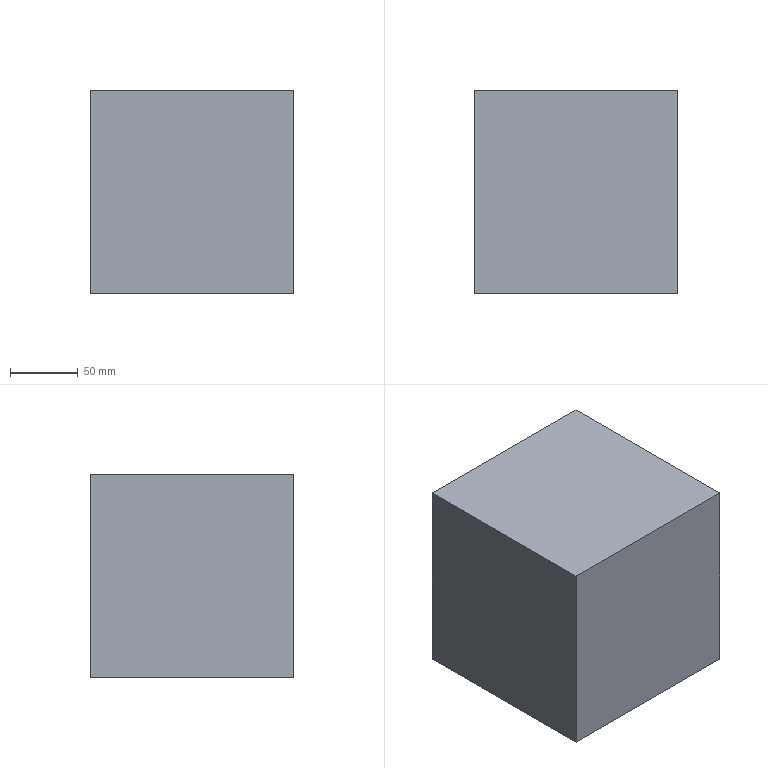Part | STEP file | Collection box | 1 solid | 11 faces | box 150 x 150 x 150 mm | volume 220232 mm3 | plane 11
STEP:
#1=CARTESIAN_POINT('',(75.,75.,-75.));
#2=VERTEX_POINT('',#1);
#3=CARTESIAN_POINT('',(-75.,75.,-75.));
#4=VERTEX_POINT('',#3);
#5=CARTESIAN_POINT('',(-75.,75.,-75.));
#6=DIRECTION('',(-1.,0.,0.));
#7=VECTOR('',#6,1000.);
#8=LINE('',#5,#7);
#9=EDGE_CURVE('',#2,#4,#8,.T.);
#10=ORIENTED_EDGE('',*,*,#9,.T.);
#11=CARTESIAN_POINT('',(-75.,75.,75.));
#12=VERTEX_POINT('',#11);
#13=CARTESIAN_POINT('',(-75.,75.,75.));
#14=DIRECTION('',(0.,0.,-1.));
#15=VECTOR('',#14,1000.);
#16=LINE('',#13,#15);
#17=EDGE_CURVE('',#12,#4,#16,.T.);
#18=ORIENTED_EDGE('',*,*,#17,.F.);
#19=CARTESIAN_POINT('',(75.,75.,75.));
#20=VERTEX_POINT('',#19);
#21=CARTESIAN_POINT('',(-75.,75.,75.));
#22=DIRECTION('',(-1.,0.,0.));
#23=VECTOR('',#22,1000.);
#24=LINE('',#21,#23);
#25=EDGE_CURVE('',#20,#12,#24,.T.);
#26=ORIENTED_EDGE('',*,*,#25,.F.);
#27=CARTESIAN_POINT('',(75.,75.,75.));
#28=DIRECTION('',(0.,0.,-1.));
#29=VECTOR('',#28,1000.);
#30=LINE('',#27,#29);
#31=EDGE_CURVE('',#20,#2,#30,.T.);
#32=ORIENTED_EDGE('',*,*,#31,.T.);
#33=EDGE_LOOP('',(#10,#18,#26,#32));
#34=FACE_OUTER_BOUND('',#33,.T.);
#35=CARTESIAN_POINT('',(73.,75.,-73.));
#36=VERTEX_POINT('',#35);
#37=CARTESIAN_POINT('',(-73.,75.,-73.));
#38=VERTEX_POINT('',#37);
#39=CARTESIAN_POINT('',(0.,75.,-73.));
#40=DIRECTION('',(-1.,0.,0.));
#41=VECTOR('',#40,1000.);
#42=LINE('',#39,#41);
#43=EDGE_CURVE('',#36,#38,#42,.T.);
#44=ORIENTED_EDGE('',*,*,#43,.F.);
#45=CARTESIAN_POINT('',(73.,75.,73.));
#46=VERTEX_POINT('',#45);
#47=CARTESIAN_POINT('',(73.,75.,75.));
#48=DIRECTION('',(0.,0.,-1.));
#49=VECTOR('',#48,1000.);
#50=LINE('',#47,#49);
#51=EDGE_CURVE('',#46,#36,#50,.T.);
#52=ORIENTED_EDGE('',*,*,#51,.F.);
#53=CARTESIAN_POINT('',(-73.,75.,73.));
#54=VERTEX_POINT('',#53);
#55=CARTESIAN_POINT('',(0.,75.,73.));
#56=DIRECTION('',(-1.,0.,0.));
#57=VECTOR('',#56,1000.);
#58=LINE('',#55,#57);
#59=EDGE_CURVE('',#46,#54,#58,.T.);
#60=ORIENTED_EDGE('',*,*,#59,.T.);
#61=CARTESIAN_POINT('',(-73.,75.,75.));
#62=DIRECTION('',(0.,0.,-1.));
#63=VECTOR('',#62,1000.);
#64=LINE('',#61,#63);
#65=EDGE_CURVE('',#54,#38,#64,.T.);
#66=ORIENTED_EDGE('',*,*,#65,.T.);
#67=EDGE_LOOP('',(#44,#52,#60,#66));
#68=FACE_BOUND('',#67,.T.);
#69=CARTESIAN_POINT('',(-75.,75.,75.));
#70=DIRECTION('',(0.,-1.,0.));
#71=DIRECTION('',(0.,0.,-1.));
#72=AXIS2_PLACEMENT_3D('',#69,#70,#71);
#73=PLANE('',#72);
#74=ADVANCED_FACE('',(#34,#68),#73,.F.);
#75=CARTESIAN_POINT('',(75.,-75.,-75.));
#76=VERTEX_POINT('',#75);
#77=CARTESIAN_POINT('',(75.,-75.,-75.));
#78=DIRECTION('',(0.,1.,0.));
#79=VECTOR('',#78,1000.);
#80=LINE('',#77,#79);
#81=EDGE_CURVE('',#76,#2,#80,.T.);
#82=ORIENTED_EDGE('',*,*,#81,.T.);
#83=ORIENTED_EDGE('',*,*,#31,.F.);
#84=CARTESIAN_POINT('',(75.,-75.,75.));
#85=VERTEX_POINT('',#84);
#86=CARTESIAN_POINT('',(75.,-75.,75.));
#87=DIRECTION('',(0.,1.,0.));
#88=VECTOR('',#87,1000.);
#89=LINE('',#86,#88);
#90=EDGE_CURVE('',#85,#20,#89,.T.);
#91=ORIENTED_EDGE('',*,*,#90,.F.);
#92=CARTESIAN_POINT('',(75.,-75.,75.));
#93=DIRECTION('',(0.,0.,-1.));
#94=VECTOR('',#93,1000.);
#95=LINE('',#92,#94);
#96=EDGE_CURVE('',#85,#76,#95,.T.);
#97=ORIENTED_EDGE('',*,*,#96,.T.);
#98=EDGE_LOOP('',(#82,#83,#91,#97));
#99=FACE_OUTER_BOUND('',#98,.T.);
#100=CARTESIAN_POINT('',(75.,-75.,75.));
#101=DIRECTION('',(-1.,0.,0.));
#102=DIRECTION('',(0.,0.,1.));
#103=AXIS2_PLACEMENT_3D('',#100,#101,#102);
#104=PLANE('',#103);
#105=ADVANCED_FACE('',(#99),#104,.F.);
#106=CARTESIAN_POINT('',(-75.,-75.,-75.));
#107=VERTEX_POINT('',#106);
#108=CARTESIAN_POINT('',(-75.,-75.,-75.));
#109=DIRECTION('',(0.,-1.,0.));
#110=VECTOR('',#109,1000.);
#111=LINE('',#108,#110);
#112=EDGE_CURVE('',#4,#107,#111,.T.);
#113=ORIENTED_EDGE('',*,*,#112,.T.);
#114=CARTESIAN_POINT('',(-75.,-75.,75.));
#115=VERTEX_POINT('',#114);
#116=CARTESIAN_POINT('',(-75.,-75.,75.));
#117=DIRECTION('',(0.,0.,-1.));
#118=VECTOR('',#117,1000.);
#119=LINE('',#116,#118);
#120=EDGE_CURVE('',#115,#107,#119,.T.);
#121=ORIENTED_EDGE('',*,*,#120,.F.);
#122=CARTESIAN_POINT('',(-75.,-75.,75.));
#123=DIRECTION('',(0.,-1.,0.));
#124=VECTOR('',#123,1000.);
#125=LINE('',#122,#124);
#126=EDGE_CURVE('',#12,#115,#125,.T.);
#127=ORIENTED_EDGE('',*,*,#126,.F.);
#128=ORIENTED_EDGE('',*,*,#17,.T.);
#129=EDGE_LOOP('',(#113,#121,#127,#128));
#130=FACE_OUTER_BOUND('',#129,.T.);
#131=CARTESIAN_POINT('',(-75.,-75.,75.));
#132=DIRECTION('',(1.,0.,0.));
#133=DIRECTION('',(0.,0.,-1.));
#134=AXIS2_PLACEMENT_3D('',#131,#132,#133);
#135=PLANE('',#134);
#136=ADVANCED_FACE('',(#130),#135,.F.);
#137=CARTESIAN_POINT('',(-75.,-75.,-75.));
#138=DIRECTION('',(1.,0.,0.));
#139=VECTOR('',#138,1000.);
#140=LINE('',#137,#139);
#141=EDGE_CURVE('',#107,#76,#140,.T.);
#142=ORIENTED_EDGE('',*,*,#141,.T.);
#143=ORIENTED_EDGE('',*,*,#96,.F.);
#144=CARTESIAN_POINT('',(-75.,-75.,75.));
#145=DIRECTION('',(1.,0.,0.));
#146=VECTOR('',#145,1000.);
#147=LINE('',#144,#146);
#148=EDGE_CURVE('',#115,#85,#147,.T.);
#149=ORIENTED_EDGE('',*,*,#148,.F.);
#150=ORIENTED_EDGE('',*,*,#120,.T.);
#151=EDGE_LOOP('',(#142,#143,#149,#150));
#152=FACE_OUTER_BOUND('',#151,.T.);
#153=CARTESIAN_POINT('',(-75.,-75.,75.));
#154=DIRECTION('',(0.,1.,0.));
#155=DIRECTION('',(0.,0.,1.));
#156=AXIS2_PLACEMENT_3D('',#153,#154,#155);
#157=PLANE('',#156);
#158=ADVANCED_FACE('',(#152),#157,.F.);
#159=ORIENTED_EDGE('',*,*,#90,.T.);
#160=ORIENTED_EDGE('',*,*,#25,.T.);
#161=ORIENTED_EDGE('',*,*,#126,.T.);
#162=ORIENTED_EDGE('',*,*,#148,.T.);
#163=EDGE_LOOP('',(#159,#160,#161,#162));
#164=FACE_OUTER_BOUND('',#163,.T.);
#165=CARTESIAN_POINT('',(0.,0.,75.));
#166=DIRECTION('',(0.,0.,-1.));
#167=DIRECTION('',(-1.,0.,0.));
#168=AXIS2_PLACEMENT_3D('',#165,#166,#167);
#169=PLANE('',#168);
#170=ADVANCED_FACE('',(#164),#169,.F.);
#171=ORIENTED_EDGE('',*,*,#81,.F.);
#172=ORIENTED_EDGE('',*,*,#141,.F.);
#173=ORIENTED_EDGE('',*,*,#112,.F.);
#174=ORIENTED_EDGE('',*,*,#9,.F.);
#175=EDGE_LOOP('',(#171,#172,#173,#174));
#176=FACE_OUTER_BOUND('',#175,.T.);
#177=CARTESIAN_POINT('',(0.,0.,-75.));
#178=DIRECTION('',(0.,0.,-1.));
#179=DIRECTION('',(-1.,0.,0.));
#180=AXIS2_PLACEMENT_3D('',#177,#178,#179);
#181=PLANE('',#180);
#182=ADVANCED_FACE('',(#176),#181,.T.);
#183=CARTESIAN_POINT('',(73.,-73.,-73.));
#184=VERTEX_POINT('',#183);
#185=CARTESIAN_POINT('',(73.,0.,-73.));
#186=DIRECTION('',(0.,1.,0.));
#187=VECTOR('',#186,1000.);
#188=LINE('',#185,#187);
#189=EDGE_CURVE('',#184,#36,#188,.T.);
#190=ORIENTED_EDGE('',*,*,#189,.F.);
#191=CARTESIAN_POINT('',(73.,-73.,73.));
#192=VERTEX_POINT('',#191);
#193=CARTESIAN_POINT('',(73.,-73.,75.));
#194=DIRECTION('',(0.,0.,-1.));
#195=VECTOR('',#194,1000.);
#196=LINE('',#193,#195);
#197=EDGE_CURVE('',#192,#184,#196,.T.);
#198=ORIENTED_EDGE('',*,*,#197,.F.);
#199=CARTESIAN_POINT('',(73.,0.,73.));
#200=DIRECTION('',(0.,1.,0.));
#201=VECTOR('',#200,1000.);
#202=LINE('',#199,#201);
#203=EDGE_CURVE('',#192,#46,#202,.T.);
#204=ORIENTED_EDGE('',*,*,#203,.T.);
#205=ORIENTED_EDGE('',*,*,#51,.T.);
#206=EDGE_LOOP('',(#190,#198,#204,#205));
#207=FACE_OUTER_BOUND('',#206,.T.);
#208=CARTESIAN_POINT('',(73.,-75.,75.));
#209=DIRECTION('',(-1.,0.,0.));
#210=DIRECTION('',(0.,0.,1.));
#211=AXIS2_PLACEMENT_3D('',#208,#209,#210);
#212=PLANE('',#211);
#213=ADVANCED_FACE('',(#207),#212,.T.);
#214=CARTESIAN_POINT('',(-73.,-73.,-73.));
#215=VERTEX_POINT('',#214);
#216=CARTESIAN_POINT('',(-73.,0.,-73.));
#217=DIRECTION('',(0.,-1.,0.));
#218=VECTOR('',#217,1000.);
#219=LINE('',#216,#218);
#220=EDGE_CURVE('',#38,#215,#219,.T.);
#221=ORIENTED_EDGE('',*,*,#220,.F.);
#222=ORIENTED_EDGE('',*,*,#65,.F.);
#223=CARTESIAN_POINT('',(-73.,-73.,73.));
#224=VERTEX_POINT('',#223);
#225=CARTESIAN_POINT('',(-73.,0.,73.));
#226=DIRECTION('',(0.,-1.,0.));
#227=VECTOR('',#226,1000.);
#228=LINE('',#225,#227);
#229=EDGE_CURVE('',#54,#224,#228,.T.);
#230=ORIENTED_EDGE('',*,*,#229,.T.);
#231=CARTESIAN_POINT('',(-73.,-73.,75.));
#232=DIRECTION('',(0.,0.,-1.));
#233=VECTOR('',#232,1000.);
#234=LINE('',#231,#233);
#235=EDGE_CURVE('',#224,#215,#234,.T.);
#236=ORIENTED_EDGE('',*,*,#235,.T.);
#237=EDGE_LOOP('',(#221,#222,#230,#236));
#238=FACE_OUTER_BOUND('',#237,.T.);
#239=CARTESIAN_POINT('',(-73.,-75.,75.));
#240=DIRECTION('',(1.,0.,0.));
#241=DIRECTION('',(0.,0.,-1.));
#242=AXIS2_PLACEMENT_3D('',#239,#240,#241);
#243=PLANE('',#242);
#244=ADVANCED_FACE('',(#238),#243,.T.);
#245=CARTESIAN_POINT('',(0.,-73.,-73.));
#246=DIRECTION('',(1.,0.,0.));
#247=VECTOR('',#246,1000.);
#248=LINE('',#245,#247);
#249=EDGE_CURVE('',#215,#184,#248,.T.);
#250=ORIENTED_EDGE('',*,*,#249,.F.);
#251=ORIENTED_EDGE('',*,*,#235,.F.);
#252=CARTESIAN_POINT('',(0.,-73.,73.));
#253=DIRECTION('',(1.,0.,0.));
#254=VECTOR('',#253,1000.);
#255=LINE('',#252,#254);
#256=EDGE_CURVE('',#224,#192,#255,.T.);
#257=ORIENTED_EDGE('',*,*,#256,.T.);
#258=ORIENTED_EDGE('',*,*,#197,.T.);
#259=EDGE_LOOP('',(#250,#251,#257,#258));
#260=FACE_OUTER_BOUND('',#259,.T.);
#261=CARTESIAN_POINT('',(-75.,-73.,75.));
#262=DIRECTION('',(0.,1.,0.));
#263=DIRECTION('',(0.,0.,1.));
#264=AXIS2_PLACEMENT_3D('',#261,#262,#263);
#265=PLANE('',#264);
#266=ADVANCED_FACE('',(#260),#265,.T.);
#267=ORIENTED_EDGE('',*,*,#203,.F.);
#268=ORIENTED_EDGE('',*,*,#256,.F.);
#269=ORIENTED_EDGE('',*,*,#229,.F.);
#270=ORIENTED_EDGE('',*,*,#59,.F.);
#271=EDGE_LOOP('',(#267,#268,#269,#270));
#272=FACE_OUTER_BOUND('',#271,.T.);
#273=CARTESIAN_POINT('',(0.,0.,73.));
#274=DIRECTION('',(0.,0.,-1.));
#275=DIRECTION('',(-1.,0.,0.));
#276=AXIS2_PLACEMENT_3D('',#273,#274,#275);
#277=PLANE('',#276);
#278=ADVANCED_FACE('',(#272),#277,.T.);
#279=ORIENTED_EDGE('',*,*,#189,.T.);
#280=ORIENTED_EDGE('',*,*,#43,.T.);
#281=ORIENTED_EDGE('',*,*,#220,.T.);
#282=ORIENTED_EDGE('',*,*,#249,.T.);
#283=EDGE_LOOP('',(#279,#280,#281,#282));
#284=FACE_OUTER_BOUND('',#283,.T.);
#285=CARTESIAN_POINT('',(0.,0.,-73.));
#286=DIRECTION('',(0.,0.,-1.));
#287=DIRECTION('',(-1.,0.,0.));
#288=AXIS2_PLACEMENT_3D('',#285,#286,#287);
#289=PLANE('',#288);
#290=ADVANCED_FACE('',(#284),#289,.F.);
#291=CLOSED_SHELL('',(#74,#105,#136,#158,#170,#182,#213,#244,#266,#278,#290));
#292=MANIFOLD_SOLID_BREP('',#291);
#293=CARTESIAN_POINT('',(0.,0.,0.));
#294=DIRECTION('',(0.,0.,1.));
#295=DIRECTION('',(1.,0.,0.));
#296=AXIS2_PLACEMENT_3D('',#293,#294,#295);
#297=(LENGTH_UNIT()NAMED_UNIT(*)SI_UNIT(.MILLI.,.METRE.));
#298=UNCERTAINTY_MEASURE_WITH_UNIT(LENGTH_MEASURE(0.00001),#297,'','');
#299=(NAMED_UNIT(*)PLANE_ANGLE_UNIT()SI_UNIT($,.RADIAN.));
#300=(NAMED_UNIT(*)SI_UNIT($,.STERADIAN.)SOLID_ANGLE_UNIT());
#301=(GEOMETRIC_REPRESENTATION_CONTEXT(3)GLOBAL_UNCERTAINTY_ASSIGNED_CONTEXT((#298))GLOBAL_UNIT_ASSIGNED_CONTEXT((#297,#299,#300))REPRESENTATION_CONTEXT('',''));
#302=ADVANCED_BREP_SHAPE_REPRESENTATION('',(#292,#296),#301);